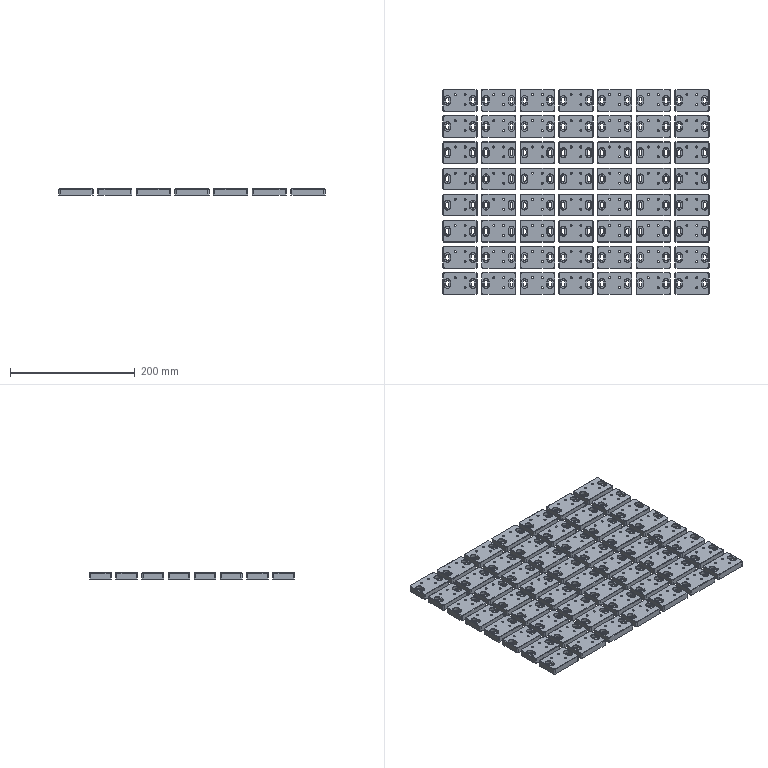NC program | NX | posted with a generic post | part box 427 x 329 x 10 mm
Whole program:
N10 G17 G21 G94 G90
(DRILLING_COPY , TOOL : D4A45)
N12 T02 M6
N14 G54
N16 G17 G0 G90 X7.95 Y-6.65 S5000 M3
N18 G43 Z30. H2
N20 G94 G81 G98 Z-1. F250. R3.
N22 Y9.25
N24 X-7.95
N26 G80
N28 G0 X-7.95 Y9.25 Z30.
N30 M5
(DRILLING_COPY_COPY_COPY_COPY_COPY_COPY_1 , TOOL : 3.3ZT)
N32 T13 M6
N34 G54
N36 G17 G0 G90 X7.95 Y-6.65 S1910 M3
N38 G43 Z30. H13
N40 G94 G83 G98 Z-12.431 F180. Q2. R3.
N42 Y9.25
N44 X-7.95
N46 G80
N48 G0 X-7.95 Y9.25 Z30.
N50 M5
(ZLEVEL_PROFILE_COPY_COPY_1_COPY_COPY , TOOL : D6)
N52 T06 M6
N54 G54
N56 G17 G0 G90 X-21.089 Y-4.308 S9500 M3
N58 G43 Z30. H6
N60 Z1.5
N62 G94 G1 X-20.501 Y-4.43 Z1.469 F1000.
N64 X-19.836 Y-4.293 Z1.433
N66 X-19.28 Y-3.905 Z1.397
N68 X-18.939 Y-3.372 Z1.364
N70 X-18.85 Y-3.066 Z1.348
N72 Y2.75 Z1.043
N74 X-18.873 Y2.784 Z1.041
N76 X-18.893 Y2.99 Z1.03
N78 X-18.937 Y3.301 Z1.013
N80 X-19.208 Y3.794 Z0.984
N82 X-19.627 Y4.168 Z0.954
N84 X-20.213 Y4.396 Z0.921
N86 X-20.939 Y4.367 Z0.883
N88 X-21.584 Y4.031 Z0.845
N90 X-22.024 Y3.453 Z0.807
N92 X-22.099 Y3.148 Z0.791
N94 X-22.135 Y2.767 Z0.771
N96 X-22.15 Z0.77
N98 Y-3.066 Z0.464
N100 X-22.061 Y-3.37 Z0.448
N102 X-21.722 Y-3.903 Z0.414
N104 X-21.166 Y-4.292 Z0.379
N106 X-20.501 Y-4.43 Z0.343
N108 X-19.836 Y-4.293 Z0.308
N110 X-19.28 Y-3.905 Z0.272
N112 X-18.939 Y-3.372 Z0.239
N114 X-18.85 Y-3.066 Z0.222
N116 Y2.75 Z-0.082
N118 X-18.873 Y2.784 Z-0.085
N120 X-18.893 Y2.99 Z-0.095
N122 X-18.937 Y3.301 Z-0.112
N124 X-19.208 Y3.794 Z-0.141
N126 X-19.627 Y4.168 Z-0.171
N128 X-20.213 Y4.396 Z-0.204
N130 X-20.939 Y4.367 Z-0.242
N132 X-21.584 Y4.031 Z-0.28
N134 X-22.024 Y3.453 Z-0.318
N136 X-22.099 Y3.148 Z-0.335
N138 X-22.135 Y2.767 Z-0.355
N140 X-22.15
N142 Y0.008 Z-0.5
N144 Y-2.75 F2200.
N146 G3 X-20.5 Y-4.4 R1.65
N148 X-18.85 Y-2.75 R1.65
N150 G1 Y2.75
N152 X-18.873 Y2.784
N154 X-18.893 Y2.99
N156 G3 X-22.099 Y3.148 R1.635
N158 G1 X-22.135 Y2.767
N160 X-22.15
N162 Y0.008
N164 Y-2.365 Z-0.574
N166 Y-2.661 Z-0.583
N168 X-22.112 Y-2.954 Z-0.593
N170 X-22.018 Y-3.341 Z-0.605
N172 X-21.944 Y-3.512 Z-0.611
N174 X-21.744 Y-3.812 Z-0.622
N176 X-21.59 Y-3.978 Z-0.63
N178 X-21.326 Y-4.169 Z-0.64
N180 X-21.087 Y-4.281 Z-0.648
N182 X-20.743 Y-4.374 Z-0.659
N184 X-20.511 Y-4.394 Z-0.667
N186 X-20.181 Y-4.361 Z-0.677
N188 X-19.934 Y-4.288 Z-0.685
N190 X-19.613 Y-4.127 Z-0.696
N192 X-19.427 Y-3.993 Z-0.704
N194 X-19.203 Y-3.755 Z-0.714
N196 X-19.156 Y-3.681 Z-0.717
N198 X-19.067 Y-3.531 Z-0.722
N200 X-18.954 Y-3.256 Z-0.732
N202 X-18.891 Y-2.976 Z-0.741
N204 X-18.86 Y-2.682 Z-0.75
N206 X-18.85 Y-2.387 Z-0.759
N208 Y2.359 Z-0.907
N210 Y2.653 Z-0.917
N212 X-18.889 Y2.945 Z-0.926
N214 X-18.986 Y3.352 Z-0.939
N216 X-19.055 Y3.511 Z-0.944
N218 X-19.254 Y3.81 Z-0.956
N220 X-19.416 Y3.981 Z-0.963
N222 X-19.683 Y4.171 Z-0.973
N224 X-19.923 Y4.283 Z-0.981
N226 X-20.209 Y4.364 Z-0.991
N228 X-20.503 Y4.4 Z-1.
N230 G3 X-22.15 Y2.75 R1.65
N232 G1 Y0.008
N234 Y-2.366 Z-1.074
N236 Y-2.662 Z-1.083
N238 X-22.112 Y-2.956 Z-1.093
N240 X-22.018 Y-3.342 Z-1.105
N242 X-21.943 Y-3.513 Z-1.111
N244 X-21.743 Y-3.813 Z-1.122
N246 X-21.588 Y-3.979 Z-1.13
N248 X-21.325 Y-4.168 Z-1.14
N250 X-21.085 Y-4.282 Z-1.148
N252 X-20.736 Y-4.376 Z-1.159
N254 X-20.508 Y-4.396 Z-1.167
N256 X-20.184 Y-4.362 Z-1.177
N258 X-19.931 Y-4.287 Z-1.185
N260 X-19.61 Y-4.125 Z-1.196
N262 X-19.424 Y-3.99 Z-1.204
N264 X-19.274 Y-3.833 Z-1.211
N266 X-19.199 Y-3.753 Z-1.214
N268 X-19.065 Y-3.528 Z-1.222
N270 X-18.952 Y-3.255 Z-1.232
N272 X-18.89 Y-2.972 Z-1.241
N274 X-18.86 Y-2.678 Z-1.25
N276 X-18.85 Y-2.382 Z-1.259
N278 Y2.366 Z-1.407
N280 Y2.662 Z-1.417
N282 X-18.888 Y2.956 Z-1.426
N284 X-18.984 Y3.344 Z-1.439
N286 X-19.057 Y3.513 Z-1.444
N288 X-19.253 Y3.808 Z-1.456
N290 X-19.414 Y3.977 Z-1.463
N292 X-19.681 Y4.17 Z-1.473
N294 X-19.915 Y4.281 Z-1.481
N296 X-20.199 Y4.363 Z-1.491
N298 X-20.492 Y4.4 Z-1.5
N300 G3 X-22.15 Y2.75 R1.65
N302 G1 Y0.008
N304 Y-2.366 Z-1.574
N306 Y-2.662 Z-1.583
N308 X-22.112 Y-2.956 Z-1.593
N310 X-22.017 Y-3.342 Z-1.605
N312 X-21.943 Y-3.513 Z-1.611
N314 X-21.743 Y-3.812 Z-1.622
N316 X-21.588 Y-3.979 Z-1.63
N318 X-21.326 Y-4.168 Z-1.64
N320 X-21.085 Y-4.281 Z-1.648
N322 X-20.737 Y-4.376 Z-1.659
N324 X-20.508 Y-4.396 Z-1.667
N326 X-20.184 Y-4.362 Z-1.677
N328 X-19.931 Y-4.287 Z-1.685
N330 X-19.61 Y-4.124 Z-1.696
N332 X-19.424 Y-3.99 Z-1.704
N334 X-19.274 Y-3.833 Z-1.711
N336 X-19.2 Y-3.753 Z-1.714
N338 X-19.065 Y-3.528 Z-1.722
N340 X-18.952 Y-3.255 Z-1.732
N342 X-18.891 Y-2.972 Z-1.741
N344 X-18.86 Y-2.678 Z-1.75
N346 X-18.85 Y-2.382 Z-1.759
N348 Y2.366 Z-1.907
N350 Y2.662 Z-1.917
N352 X-18.888 Y2.956 Z-1.926
N354 X-18.984 Y3.344 Z-1.939
N356 X-19.058 Y3.513 Z-1.944
N358 X-19.253 Y3.808 Z-1.956
N360 X-19.414 Y3.977 Z-1.963
N362 X-19.681 Y4.17 Z-1.973
N364 X-19.915 Y4.281 Z-1.981
N366 X-20.199 Y4.362 Z-1.991
N368 X-20.492 Y4.4 Z-2.
N370 G3 X-22.15 Y2.75 R1.65
N372 G1 Y0.008
N374 Y-2.366 Z-2.074
N376 Y-2.662 Z-2.083
N378 X-22.112 Y-2.956 Z-2.093
N380 X-22.017 Y-3.343 Z-2.105
N382 X-21.942 Y-3.513 Z-2.111
N384 X-21.745 Y-3.813 Z-2.122
N386 X-21.588 Y-3.979 Z-2.13
N388 X-21.321 Y-4.17 Z-2.14
N390 X-21.085 Y-4.281 Z-2.148
N392 X-20.736 Y-4.375 Z-2.159
N394 X-20.508 Y-4.396 Z-2.167
N396 X-20.185 Y-4.362 Z-2.177
N398 X-19.931 Y-4.287 Z-2.185
N400 X-19.611 Y-4.124 Z-2.196
N402 X-19.425 Y-3.99 Z-2.204
N404 X-19.275 Y-3.833 Z-2.211
N406 X-19.2 Y-3.754 Z-2.214
N408 X-19.065 Y-3.527 Z-2.222
N410 X-18.953 Y-3.255 Z-2.232
N412 X-18.891 Y-2.972 Z-2.241
N414 X-18.86 Y-2.678 Z-2.25
N416 X-18.85 Y-2.382 Z-2.259
N418 Y2.366 Z-2.407
N420 Y2.662 Z-2.417
N422 X-18.889 Y2.956 Z-2.426
N424 X-18.985 Y3.345 Z-2.439
N426 X-19.058 Y3.513 Z-2.444
N428 X-19.253 Y3.807 Z-2.456
N430 X-19.414 Y3.977 Z-2.463
N432 X-19.681 Y4.169 Z-2.473
N434 X-19.915 Y4.281 Z-2.481
N436 X-20.2 Y4.362 Z-2.491
N438 X-20.492 Y4.4 Z-2.5
N440 G3 X-22.15 Y2.75 R1.65
N442 G1 Y0.008
N444 Y-2.366 Z-2.574
N446 Y-2.662 Z-2.583
N448 X-22.112 Y-2.956 Z-2.593
N450 X-22.018 Y-3.344 Z-2.605
N452 X-21.942 Y-3.513 Z-2.611
N454 X-21.738 Y-3.817 Z-2.623
N456 X-21.588 Y-3.979 Z-2.63
N458 X-21.325 Y-4.168 Z-2.64
N460 X-21.085 Y-4.281 Z-2.648
N462 X-20.737 Y-4.375 Z-2.659
N464 X-20.508 Y-4.396 Z-2.667
N466 X-20.185 Y-4.362 Z-2.677
N468 X-19.931 Y-4.287 Z-2.685
N470 X-19.612 Y-4.124 Z-2.696
N472 X-19.425 Y-3.99 Z-2.704
N474 X-19.2 Y-3.754 Z-2.714
N476 X-19.066 Y-3.527 Z-2.722
N478 X-18.953 Y-3.255 Z-2.732
N480 X-18.891 Y-2.972 Z-2.741
N482 X-18.86 Y-2.678 Z-2.75
N484 X-18.85 Y-2.382 Z-2.759
N486 Y2.366 Z-2.907
N488 Y2.662 Z-2.917
N490 X-18.889 Y2.956 Z-2.926
N492 X-18.985 Y3.345 Z-2.939
N494 X-19.058 Y3.513 Z-2.944
N496 X-19.253 Y3.807 Z-2.956
N498 X-19.414 Y3.977 Z-2.963
N500 X-19.68 Y4.169 Z-2.973
N502 X-19.916 Y4.281 Z-2.981
N504 X-20.2 Y4.362 Z-2.991
N506 X-20.492 Y4.4 Z-3.
N508 G3 X-22.15 Y2.75 R1.65
N510 G1 Y0.008
N512 Y-2.366 Z-3.074
N514 Y-2.662 Z-3.083
N516 X-22.111 Y-2.956 Z-3.093
N518 X-22.018 Y-3.344 Z-3.105
N520 X-21.942 Y-3.513 Z-3.111
N522 X-21.738 Y-3.816 Z-3.123
N524 X-21.588 Y-3.979 Z-3.13
N526 X-21.325 Y-4.167 Z-3.14
N528 X-21.085 Y-4.281 Z-3.148
N530 X-20.738 Y-4.374 Z-3.159
N532 X-20.508 Y-4.396 Z-3.167
N534 X-20.186 Y-4.361 Z-3.177
N536 X-19.931 Y-4.287 Z-3.185
N538 X-19.612 Y-4.124 Z-3.196
N540 X-19.425 Y-3.99 Z-3.204
N542 X-19.276 Y-3.833 Z-3.21
N544 X-19.203 Y-3.753 Z-3.214
N546 X-19.156 Y-3.678 Z-3.217
N548 X-19.066 Y-3.527 Z-3.222
N550 X-18.954 Y-3.258 Z-3.231
N552 X-18.891 Y-2.972 Z-3.241
N554 X-18.861 Y-2.678 Z-3.25
N556 X-18.85 Y-2.382 Z-3.259
N558 Y2.366 Z-3.407
N560 Y2.662 Z-3.417
N562 X-18.889 Y2.956 Z-3.426
N564 X-18.985 Y3.345 Z-3.439
N566 X-19.058 Y3.513 Z-3.444
N568 X-19.254 Y3.806 Z-3.456
N570 X-19.414 Y3.977 Z-3.463
N572 X-19.68 Y4.168 Z-3.473
N574 X-19.916 Y4.281 Z-3.481
N576 X-20.2 Y4.362 Z-3.491
N578 X-20.492 Y4.4 Z-3.5
N580 G3 X-22.15 Y2.75 R1.65
N582 G1 Y0.008
N584 Y-2.366 Z-3.574
N586 Y-2.662 Z-3.583
N588 X-22.111 Y-2.956 Z-3.593
N590 X-22.017 Y-3.345 Z-3.605
N592 X-21.942 Y-3.513 Z-3.611
N594 X-21.738 Y-3.816 Z-3.623
N596 X-21.587 Y-3.979 Z-3.63
N598 X-21.325 Y-4.167 Z-3.64
N600 X-21.084 Y-4.281 Z-3.648
N602 X-20.738 Y-4.374 Z-3.659
N604 X-20.508 Y-4.396 Z-3.667
N606 X-20.186 Y-4.361 Z-3.677
N608 X-19.931 Y-4.286 Z-3.685
N610 X-19.613 Y-4.124 Z-3.696
N612 X-19.425 Y-3.99 Z-3.704
N614 X-19.276 Y-3.833 Z-3.71
N616 X-19.203 Y-3.753 Z-3.714
N618 X-19.157 Y-3.678 Z-3.717
N620 X-19.066 Y-3.527 Z-3.722
N622 X-18.955 Y-3.259 Z-3.731
N624 X-18.891 Y-2.972 Z-3.741
N626 X-18.861 Y-2.678 Z-3.75
N628 X-18.85 Y-2.382 Z-3.759
N630 Y2.366 Z-3.907
N632 Y2.662 Z-3.917
N634 X-18.889 Y2.956 Z-3.926
N636 X-18.986 Y3.345 Z-3.939
N638 X-19.058 Y3.513 Z-3.944
N640 X-19.254 Y3.806 Z-3.956
N642 X-19.414 Y3.977 Z-3.963
N644 X-19.68 Y4.168 Z-3.973
N646 X-19.916 Y4.28 Z-3.981
N648 X-20.2 Y4.362 Z-3.991
N650 X-20.492 Y4.4 Z-4.
N652 G3 X-22.15 Y2.75 R1.65
N654 G1 Y0.008
N656 Y-2.366 Z-4.074
N658 Y-2.662 Z-4.083
N660 X-22.111 Y-2.956 Z-4.093
N662 X-22.017 Y-3.345 Z-4.105
N664 X-21.942 Y-3.513 Z-4.111
N666 X-21.74 Y-3.817 Z-4.123
N668 X-21.587 Y-3.979 Z-4.13
N670 X-21.321 Y-4.169 Z-4.14
N672 X-21.084 Y-4.281 Z-4.148
N674 X-20.737 Y-4.374 Z-4.159
N676 X-20.508 Y-4.395 Z-4.167
N678 X-20.186 Y-4.361 Z-4.177
N680 X-19.931 Y-4.286 Z-4.185
N682 X-19.613 Y-4.124 Z-4.196
N684 X-19.425 Y-3.99 Z-4.204
N686 X-19.277 Y-3.833 Z-4.21
N688 X-19.203 Y-3.753 Z-4.214
N690 X-19.157 Y-3.678 Z-4.217
N692 X-19.066 Y-3.527 Z-4.222
N694 X-18.955 Y-3.259 Z-4.231
N696 X-18.891 Y-2.972 Z-4.241
N698 X-18.861 Y-2.678 Z-4.25
N700 X-18.85 Y-2.382 Z-4.259
N702 Y2.366 Z-4.407
N704 Y2.662 Z-4.417
N706 X-18.889 Y2.956 Z-4.426
N708 X-18.984 Y3.347 Z-4.439
N710 X-19.058 Y3.513 Z-4.444
N712 X-19.258 Y3.811 Z-4.456
N714 X-19.414 Y3.977 Z-4.463
N716 X-19.681 Y4.168 Z-4.473
N718 X-19.916 Y4.28 Z-4.481
N720 X-20.2 Y4.361 Z-4.491
N722 X-20.492 Y4.4 Z-4.5
N724 G3 X-22.15 Y2.75 R1.65
N726 G1 Y0.008
N728 Y-2.366 Z-4.574
N730 Y-2.662 Z-4.583
N732 X-22.111 Y-2.956 Z-4.593
N734 X-22.017 Y-3.345 Z-4.605
N736 X-21.942 Y-3.513 Z-4.611
N738 X-21.74 Y-3.816 Z-4.623
N740 X-21.587 Y-3.978 Z-4.63
N742 X-21.322 Y-4.171 Z-4.64
N744 X-21.084 Y-4.28 Z-4.648
N746 X-20.733 Y-4.374 Z-4.66
N748 X-20.508 Y-4.395 Z-4.667
N750 X-20.186 Y-4.361 Z-4.677
N752 X-19.931 Y-4.286 Z-4.685
N754 X-19.614 Y-4.124 Z-4.696
N756 X-19.425 Y-3.989 Z-4.704
N758 X-19.277 Y-3.833 Z-4.71
N760 X-19.204 Y-3.754 Z-4.714
N762 X-19.158 Y-3.678 Z-4.717
N764 X-19.066 Y-3.527 Z-4.722
N766 X-18.956 Y-3.26 Z-4.731
N768 X-18.891 Y-2.972 Z-4.741
N770 X-18.861 Y-2.678 Z-4.75
N772 X-18.85 Y-2.382 Z-4.759
N774 Y2.366 Z-4.907
N776 Y2.662 Z-4.917
N778 X-18.889 Y2.955 Z-4.926
N780 X-18.985 Y3.347 Z-4.939
N782 X-19.059 Y3.513 Z-4.944
N784 X-19.258 Y3.81 Z-4.956
N786 X-19.415 Y3.976 Z-4.963
N788 X-19.68 Y4.167 Z-4.973
N790 X-19.916 Y4.28 Z-4.981
N792 X-20.2 Y4.361 Z-4.991
N794 X-20.492 Y4.4 Z-5.
N796 G3 X-22.15 Y2.75 R1.65
N798 G1 Y-2.75
N800 G3 X-20.5 Y-4.4 R1.65
N802 X-18.85 Y-2.75 R1.65
N804 G1 Y2.75
N806 G3 X-20.492 Y4.4 R1.65
N808 G1 Z-3.5
N810 G0 Z30.
N812 X21.052 Y4.293
N814 Z1.5
N816 G1 X20.787 Y4.396 Z1.485 F1000.
N818 X20.061 Y4.367 Z1.447
N820 X19.416 Y4.031 Z1.409
N822 X18.976 Y3.453 Z1.371
N824 X18.901 Y3.148 Z1.354
N826 X18.865 Y2.767 Z1.334
N828 X18.85 Z1.333
N830 Y-3.066 Z1.028
N832 X18.939 Y-3.37 Z1.011
N834 X19.278 Y-3.903 Z0.978
N836 X19.834 Y-4.292 Z0.943
N838 X20.499 Y-4.43 Z0.907
N840 X21.164 Y-4.293 Z0.871
N842 X21.72 Y-3.905 Z0.836
N844 X22.061 Y-3.372 Z0.803
N846 X22.15 Y-3.066 Z0.786
N848 Y2.75 Z0.481
N850 X22.127 Y2.784 Z0.479
N852 X22.107 Y2.99 Z0.468
N854 X22.063 Y3.301 Z0.452
N856 X21.792 Y3.794 Z0.422
N858 X21.373 Y4.168 Z0.393
N860 X20.787 Y4.396 Z0.36
N862 X20.061 Y4.367 Z0.322
N864 X19.416 Y4.031 Z0.284
N866 X18.976 Y3.453 Z0.246
N868 X18.901 Y3.148 Z0.229
N870 X18.865 Y2.767 Z0.209
N872 X18.85 Z0.208
N874 Y-3.066 Z-0.097
N876 X18.939 Y-3.37 Z-0.114
N878 X19.278 Y-3.903 Z-0.147
N880 X19.834 Y-4.292 Z-0.183
N882 X20.499 Y-4.43 Z-0.218
N884 X21.164 Y-4.293 Z-0.254
N886 X21.72 Y-3.905 Z-0.289
N888 X22.061 Y-3.372 Z-0.323
N890 X22.15 Y-3.066 Z-0.339
N892 Y0. Z-0.5
N894 Y2.75 F2200.
N896 X22.127 Y2.784
N898 X22.107 Y2.99
N900 G3 X18.901 Y3.148 R1.635
N902 G1 X18.865 Y2.767
N904 X18.85
N906 Y-2.75
N908 G3 X20.5 Y-4.4 R1.65
N910 X22.15 Y-2.75 R1.65
N912 G1 Y0.
N914 Y0.89 Z-0.528
N916 X22.149 Y1.186 Z-0.537
N918 X22.15 Y1.483 Z-0.546
N920 Y2.373 Z-0.574
N922 X22.141 Y2.666 Z-0.583
N924 X22.11 Y2.958 Z-0.593
N926 X22.02 Y3.335 Z-0.605
N928 X21.937 Y3.522 Z-0.611
N930 X21.733 Y3.821 Z-0.622
N932 X21.574 Y3.99 Z-0.63
N934 X21.307 Y4.178 Z-0.64
N936 X21.064 Y4.288 Z-0.648
N938 X20.721 Y4.375 Z-0.659
N940 X20.483 Y4.393 Z-0.667
N942 X20.257 Y4.376 Z-0.674
N944 X20.146 Y4.357 Z-0.677
N946 X20.065 Y4.336 Z-0.68
N948 X19.905 Y4.28 Z-0.685
N950 X19.576 Y4.105 Z-0.697
N952 X19.403 Y3.973 Z-0.704
N954 X19.25 Y3.808 Z-0.711
N956 X19.177 Y3.723 Z-0.714
N958 X19.049 Y3.505 Z-0.722
N960 X18.945 Y3.24 Z-0.731
N962 X18.882 Y2.944 Z-0.741
N964 X18.85 Y2.657 Z-0.75
N966 Y2.367 Z-0.759
N968 Y-2.378 Z-0.907
N970 Y-2.674 Z-0.917
N972 X18.89 Y-2.968 Z-0.926
N974 X18.984 Y-3.353 Z-0.938
N976 X19.063 Y-3.524 Z-0.944
N978 X19.269 Y-3.827 Z-0.956
N980 X19.421 Y-3.987 Z-0.963
N982 X19.683 Y-4.175 Z-0.973
N984 X19.926 Y-4.286 Z-0.981
N986 X20.21 Y-4.365 Z-0.991
N988 X20.503 Y-4.4 Z-1.
N990 G3 X22.15 Y-2.75 R1.65
N992 G1 Y0.
N994 Y2.077 Z-1.065
N996 X22.149 Y2.374 Z-1.074
N998 X22.141 Y2.67 Z-1.083
N1000 X22.111 Y2.964 Z-1.093
N1002 X22.021 Y3.33 Z-1.104
N1004 X21.939 Y3.52 Z-1.111
N1006 X21.745 Y3.81 Z-1.122
N1008 X21.58 Y3.983 Z-1.13
N1010 X21.31 Y4.176 Z-1.14
N1012 X21.077 Y4.284 Z-1.148
N1014 X20.732 Y4.373 Z-1.159
N1016 X20.5 Y4.395 Z-1.167
N1018 X20.176 Y4.361 Z-1.177
N1020 X19.922 Y4.286 Z-1.185
N1022 X19.604 Y4.121 Z-1.196
N1024 X19.416 Y3.988 Z-1.204
N1026 X19.272 Y3.833 Z-1.21
N1028 X19.201 Y3.755 Z-1.214
N1030 X19.15 Y3.68 Z-1.216
N1032 X19.059 Y3.522 Z-1.222
N1034 X18.942 Y3.234 Z-1.232
N1036 X18.885 Y2.964 Z-1.241
N1038 X18.85 Y2.67 Z-1.25
N1040 Y2.374 Z-1.259
N1042 Y-2.374 Z-1.407
N1044 Y-2.67 Z-1.417
N1046 X18.889 Y-2.964 Z-1.426
N1048 X18.983 Y-3.35 Z-1.438
N1050 X19.061 Y-3.52 Z-1.444
N1052 X19.267 Y-3.824 Z-1.456
N1054 X19.418 Y-3.985 Z-1.463
N1056 X19.68 Y-4.172 Z-1.473
N1058 X19.923 Y-4.284 Z-1.481
N1060 X20.207 Y-4.364 Z-1.491
N1062 X20.5 Y-4.4 Z-1.5
N1064 G3 X22.15 Y-2.75 R1.65
N1066 G1 Y0.
N1068 Y2.077 Z-1.565
N1070 X22.149 Y2.374 Z-1.574
N1072 X22.141 Y2.67 Z-1.583
N1074 X22.111 Y2.964 Z-1.593
N1076 X22.02 Y3.329 Z-1.604
N1078 X21.939 Y3.52 Z-1.611
N1080 X21.745 Y3.809 Z-1.622
N1082 X21.58 Y3.983 Z-1.63
N1084 X21.31 Y4.176 Z-1.64
N1086 X21.077 Y4.284 Z-1.648
N1088 X20.732 Y4.373 Z-1.659
N1090 X20.5 Y4.395 Z-1.667
N1092 X20.177 Y4.361 Z-1.677
N1094 X19.922 Y4.286 Z-1.685
N1096 X19.604 Y4.121 Z-1.696
N1098 X19.416 Y3.988 Z-1.704
N1100 X19.273 Y3.833 Z-1.71
N1102 X19.201 Y3.755 Z-1.714
N1104 X19.15 Y3.68 Z-1.716
N1106 X19.059 Y3.521 Z-1.722
N1108 X18.942 Y3.235 Z-1.732
N1110 X18.885 Y2.964 Z-1.741
N1112 X18.85 Y2.67 Z-1.75
N1114 Y2.374 Z-1.759
N1116 Y-2.374 Z-1.907
N1118 Y-2.67 Z-1.917
N1120 X18.889 Y-2.964 Z-1.926
N1122 X18.984 Y-3.35 Z-1.938
N1124 X19.061 Y-3.52 Z-1.944
N1126 X19.267 Y-3.823 Z-1.956
N1128 X19.418 Y-3.985 Z-1.963
N1130 X19.68 Y-4.172 Z-1.973
N1132 X19.923 Y-4.284 Z-1.981
N1134 X20.208 Y-4.364 Z-1.991
N1136 X20.5 Y-4.4 Z-2.
N1138 G3 X22.15 Y-2.75 R1.65
N1140 G1 Y0.
N1142 Y2.077 Z-2.065
N1144 X22.148 Y2.374 Z-2.074
N1146 X22.141 Y2.67 Z-2.083
N1148 X22.11 Y2.964 Z-2.093
N1150 X22.022 Y3.33 Z-2.104
N1152 X21.938 Y3.52 Z-2.111
N1154 X21.742 Y3.813 Z-2.122
N1156 X21.58 Y3.983 Z-2.13
N1158 X21.309 Y4.176 Z-2.14
N1160 X21.077 Y4.284 Z-2.148
N1162 X20.732 Y4.372 Z-2.159
N1164 X20.5 Y4.395 Z-2.167
N1166 X20.177 Y4.361 Z-2.177
N1168 X19.922 Y4.286 Z-2.185
N1170 X19.603 Y4.123 Z-2.196
N1172 X19.416 Y3.988 Z-2.204
N1174 X19.197 Y3.752 Z-2.214
N1176 X19.149 Y3.677 Z-2.217
N1178 X19.059 Y3.521 Z-2.222
N1180 X18.942 Y3.234 Z-2.232
N1182 X18.885 Y2.964 Z-2.241
N1184 X18.85 Y2.67 Z-2.25
N1186 Y2.374 Z-2.259
N1188 Y-2.374 Z-2.407
N1190 Y-2.67 Z-2.417
N1192 X18.889 Y-2.964 Z-2.426
N1194 X18.984 Y-3.35 Z-2.438
N1196 X19.061 Y-3.52 Z-2.444
N1198 X19.267 Y-3.823 Z-2.456
N1200 X19.419 Y-3.985 Z-2.463
N1202 X19.68 Y-4.171 Z-2.473
N1204 X19.923 Y-4.284 Z-2.481
N1206 X20.208 Y-4.364 Z-2.491
N1208 X20.5 Y-4.4 Z-2.5
N1210 G3 X22.15 Y-2.75 R1.65
N1212 G1 Y0.
N1214 Y2.077 Z-2.565
N1216 X22.148 Y2.374 Z-2.574
N1218 X22.14 Y2.67 Z-2.583
N1220 X22.11 Y2.964 Z-2.593
N1222 X22.022 Y3.33 Z-2.604
N1224 X21.938 Y3.52 Z-2.611
N1226 X21.742 Y3.813 Z-2.622
N1228 X21.58 Y3.983 Z-2.63
N1230 X21.31 Y4.175 Z-2.64
N1232 X21.077 Y4.284 Z-2.648
N1234 X20.732 Y4.372 Z-2.659
N1236 X20.5 Y4.395 Z-2.667
N1238 X20.178 Y4.361 Z-2.677
N1240 X19.922 Y4.286 Z-2.685
N1242 X19.604 Y4.123 Z-2.696
N1244 X19.416 Y3.987 Z-2.704
N1246 X19.197 Y3.753 Z-2.714
N1248 X19.149 Y3.677 Z-2.717
N1250 X19.06 Y3.521 Z-2.722
N1252 X18.943 Y3.235 Z-2.732
N1254 X18.885 Y2.964 Z-2.741
N1256 X18.85 Y2.67 Z-2.75
N1258 Y2.374 Z-2.759
N1260 Y-2.374 Z-2.907
N1262 Y-2.67 Z-2.917
N1264 X18.89 Y-2.964 Z-2.926
N1266 X18.985 Y-3.351 Z-2.939
N1268 X19.062 Y-3.52 Z-2.944
N1270 X19.267 Y-3.822 Z-2.956
N1272 X19.419 Y-3.984 Z-2.963
N1274 X19.68 Y-4.17 Z-2.973
N1276 X19.923 Y-4.284 Z-2.981
N1278 X20.208 Y-4.364 Z-2.991
N1280 X20.5 Y-4.4 Z-3.
N1282 G3 X22.15 Y-2.75 R1.65
N1284 G1 Y0.
N1286 Y2.077 Z-3.065
N1288 X22.148 Y2.374 Z-3.074
N1290 X22.14 Y2.67 Z-3.083
N1292 X22.11 Y2.964 Z-3.093
N1294 X22.021 Y3.33 Z-3.104
N1296 X21.938 Y3.52 Z-3.111
N1298 X21.742 Y3.812 Z-3.122
N1300 X21.58 Y3.982 Z-3.13
N1302 X21.402 Y4.114 Z-3.137
N1304 X21.311 Y4.176 Z-3.14
N1306 X21.237 Y4.219 Z-3.143
N1308 X21.077 Y4.284 Z-3.148
N1310 X20.701 Y4.378 Z-3.16
N1312 X20.5 Y4.395 Z-3.167
N1314 X20.172 Y4.36 Z-3.177
N1316 X19.922 Y4.286 Z-3.185
N1318 X19.603 Y4.122 Z-3.196
N1320 X19.416 Y3.987 Z-3.204
N1322 X19.198 Y3.752 Z-3.214
N1324 X19.15 Y3.677 Z-3.217
N1326 X19.06 Y3.521 Z-3.222
N1328 X18.943 Y3.236 Z-3.232
N1330 X18.885 Y2.964 Z-3.241
N1332 X18.85 Y2.67 Z-3.25
N1334 Y2.374 Z-3.259
N1336 Y-2.374 Z-3.407
N1338 Y-2.67 Z-3.417
N1340 X18.89 Y-2.964 Z-3.426
N1342 X18.985 Y-3.351 Z-3.439
N1344 X19.062 Y-3.52 Z-3.444
N1346 X19.267 Y-3.822 Z-3.456
N1348 X19.419 Y-3.984 Z-3.463
N1350 X19.679 Y-4.169 Z-3.473
N1352 X19.923 Y-4.284 Z-3.481
N1354 X20.207 Y-4.365 Z-3.491
N1356 X20.5 Y-4.4 Z-3.5
N1358 G3 X22.15 Y-2.75 R1.65
N1360 G1 Y0.
N1362 Y2.077 Z-3.565
N1364 X22.148 Y2.374 Z-3.574
N1366 X22.14 Y2.67 Z-3.583
N1368 X22.11 Y2.964 Z-3.593
N1370 X22.021 Y3.329 Z-3.604
N1372 X21.938 Y3.52 Z-3.611
N1374 X21.742 Y3.812 Z-3.622
N1376 X21.58 Y3.982 Z-3.63
N1378 X21.402 Y4.113 Z-3.637
N1380 X21.311 Y4.176 Z-3.64
N1382 X21.237 Y4.218 Z-3.643
N1384 X21.077 Y4.284 Z-3.648
N1386 X20.701 Y4.378 Z-3.66
N1388 X20.5 Y4.395 Z-3.667
N1390 X20.173 Y4.359 Z-3.677
N1392 X19.922 Y4.286 Z-3.685
N1394 X19.603 Y4.122 Z-3.696
N1396 X19.416 Y3.987 Z-3.704
N1398 X19.198 Y3.753 Z-3.714
N1400 X19.15 Y3.677 Z-3.717
N1402 X19.06 Y3.521 Z-3.722
N1404 X18.944 Y3.236 Z-3.732
N1406 X18.885 Y2.964 Z-3.741
N1408 X18.85 Y2.67 Z-3.75
N1410 Y2.374 Z-3.759
N1412 Y-2.374 Z-3.907
N1414 Y-2.67 Z-3.917
N1416 X18.89 Y-2.964 Z-3.926
N1418 X18.985 Y-3.351 Z-3.939
N1420 X19.062 Y-3.52 Z-3.944
N1422 X19.267 Y-3.821 Z-3.956
N1424 X19.419 Y-3.984 Z-3.963
N1426 X19.679 Y-4.169 Z-3.973
N1428 X19.923 Y-4.284 Z-3.981
N1430 X20.208 Y-4.364 Z-3.991
N1432 X20.5 Y-4.4 Z-4.
N1434 G3 X22.15 Y-2.75 R1.65
N1436 G1 Y0.
N1438 Y2.077 Z-4.065
N1440 X22.148 Y2.374 Z-4.074
N1442 X22.14 Y2.67 Z-4.083
N1444 X22.11 Y2.964 Z-4.093
N1446 X22.021 Y3.329 Z-4.104
N1448 X21.938 Y3.52 Z-4.111
N1450 X21.742 Y3.811 Z-4.122
N1452 X21.579 Y3.982 Z-4.13
N1454 X21.312 Y4.175 Z-4.14
N1456 X21.077 Y4.283 Z-4.148
N1458 X20.728 Y4.375 Z-4.159
N1460 X20.5 Y4.395 Z-4.167
N1462 X20.175 Y4.36 Z-4.177
N1464 X19.922 Y4.286 Z-4.185
N1466 X19.604 Y4.122 Z-4.196
N1468 X19.416 Y3.987 Z-4.204
N1470 X19.198 Y3.753 Z-4.214
N1472 X19.15 Y3.677 Z-4.217
N1474 X19.06 Y3.521 Z-4.222
N1476 X18.944 Y3.237 Z-4.232
N1478 X18.886 Y2.964 Z-4.241
N1480 X18.85 Y2.67 Z-4.25
N1482 Y2.374 Z-4.259
N1484 Y-2.374 Z-4.407
N1486 Y-2.67 Z-4.417
N1488 X18.89 Y-2.964 Z-4.426
N1490 X18.986 Y-3.352 Z-4.439
N1492 X19.062 Y-3.52 Z-4.444
N1494 X19.267 Y-3.821 Z-4.456
N1496 X19.419 Y-3.984 Z-4.463
N1498 X19.678 Y-4.17 Z-4.473
N1500 X19.923 Y-4.283 Z-4.481
N1502 X20.208 Y-4.364 Z-4.491
N1504 X20.5 Y-4.4 Z-4.5
N1506 G3 X22.15 Y-2.75 R1.65
N1508 G1 Y0.
N1510 Y2.077 Z-4.565
N1512 X22.148 Y2.374 Z-4.574
N1514 X22.14 Y2.67 Z-4.583
N1516 X22.11 Y2.964 Z-4.593
N1518 X22.021 Y3.329 Z-4.604
N1520 X21.938 Y3.52 Z-4.611
N1522 X21.742 Y3.81 Z-4.622
N1524 X21.579 Y3.982 Z-4.63
N1526 X21.312 Y4.175 Z-4.64
N1528 X21.077 Y4.283 Z-4.648
N1530 X20.729 Y4.374 Z-4.659
N1532 X20.5 Y4.395 Z-4.667
N1534 X20.175 Y4.359 Z-4.677
N1536 X19.923 Y4.285 Z-4.685
N1538 X19.605 Y4.122 Z-4.696
N1540 X19.416 Y3.987 Z-4.704
N1542 X19.271 Y3.831 Z-4.71
N1544 X19.199 Y3.753 Z-4.714
N1546 X19.151 Y3.677 Z-4.717
N1548 X19.06 Y3.521 Z-4.722
N1550 X18.945 Y3.238 Z-4.732
N1552 X18.886 Y2.964 Z-4.741
N1554 X18.85 Y2.67 Z-4.75
N1556 Y2.374 Z-4.759
N1558 Y-2.374 Z-4.907
N1560 Y-2.67 Z-4.917
N1562 X18.89 Y-2.964 Z-4.926
N1564 X18.986 Y-3.352 Z-4.939
N1566 X19.062 Y-3.52 Z-4.944
N1568 X19.265 Y-3.822 Z-4.956
N1570 X19.419 Y-3.984 Z-4.963
N1572 X19.593 Y-4.112 Z-4.97
N1574 X19.682 Y-4.173 Z-4.973
N1576 X19.758 Y-4.217 Z-4.976
N1578 X19.923 Y-4.283 Z-4.981
N1580 X20.208 Y-4.364 Z-4.991
N1582 X20.5 Y-4.4 Z-5.
N1584 G3 X22.15 Y-2.75 R1.65
N1586 G1 Y2.75
N1588 G3 X20.5 Y4.4 R1.65
N1590 X18.85 Y2.75 R1.65
N1592 G1 Y-2.75
N1594 G3 X20.5 Y-4.4 R1.65
N1596 G1 Z-3.5
N1598 G0 Z30.
(ZLEVEL_PROFILE_1_COPY_1_COPY_COPY_COPY , TOOL : D4A45)
N1600 T02 M6
N1602 G17 G43 G0 G90 X-23.912 Y3.488 Z30. S9500 H2 M3
N1604 Z0.
N1606 G94 G1 Z-1. F1000.
N1608 X-24.591 Y3.096
N1610 G3 X-24.791 Y2.75 R0.4
N1612 G1 Y-2.75
N1614 G3 X-20.5 Y-7.041 R4.291
N1616 X-16.209 Y-2.75 R4.291
N1618 G1 Y2.75
N1620 G3 X-20.5 Y7.041 R4.291
N1622 X-24.791 Y2.75 R4.291
N1624 X-24.591 Y2.404 R0.4
N1626 G1 X-23.991 Y2.057
N1628 Z0.
N1630 G0 Z30.
N1632 X7.95 Y9.941
N1634 Z1.
N1636 G1 Z-1.
N1638 G3 X7.259 Y9.25 R0.691
N1640 X7.95 Y9.941 R-0.691
N1642 X7.604 Y9.741 R0.4
N1644 G1 Z0.
N1646 G0 Z30.
N1648 X7.95 Y-7.341
N1650 Z1.
N1652 G1 Z-1.
N1654 G3 X8.641 Y-6.65 R0.691
N1656 X7.95 Y-7.341 R-0.691
N1658 X8.296 Y-7.141 R0.4
N1660 G1 Z0.
N1662 G0 Z30.
N1664 X23.912 Y-3.488
N1666 Z0.
N1668 G1 Z-1.
N1670 X24.591 Y-3.096
N1672 G3 X24.791 Y-2.75 R0.4
N1674 G1 Y2.75
N1676 G3 X20.5 Y7.041 R4.291
N1678 X16.209 Y2.75 R4.291
N1680 G1 Y-2.75
N1682 G3 X20.5 Y-7.041 R4.291
N1684 X24.791 Y-2.75 R4.291
N1686 X24.591 Y-2.404 R0.4
N1688 G1 X23.991 Y-2.057
N1690 Z0.
N1692 G0 Z30.
N1694 X-7.95 Y9.941
N1696 Z1.
N1698 G1 Z-1.
N1700 G3 X-8.641 Y9.25 R0.691
N1702 X-7.95 Y9.941 R-0.691
N1704 X-8.296 Y9.741 R0.4
N1706 G1 Z0.
N1708 G0 Z30.
N1710 X-26.155 Y18.692
N1712 Z0.
N1714 G1 Z-1.
N1716 X-25.846 Y18.159
N1718 G3 X-25.5 Y17.959 R0.4
N1720 G1 X25.5
N1722 G2 X27.959 Y15.5 R2.459
N1724 G1 Y-15.5
N1726 G2 X25.5 Y-17.959 R2.459
N1728 G1 X-25.5
N1730 G2 X-27.959 Y-15.5 R2.459
N1732 G1 Y15.5
N1734 G2 X-25.5 Y17.959 R2.459
N1736 G3 X-25.154 Y18.159 R0.4
N1738 G1 X-24.807 Y18.759
N1740 Z0.
N1742 G0 Z30.
N1744 M5
N1746 M2